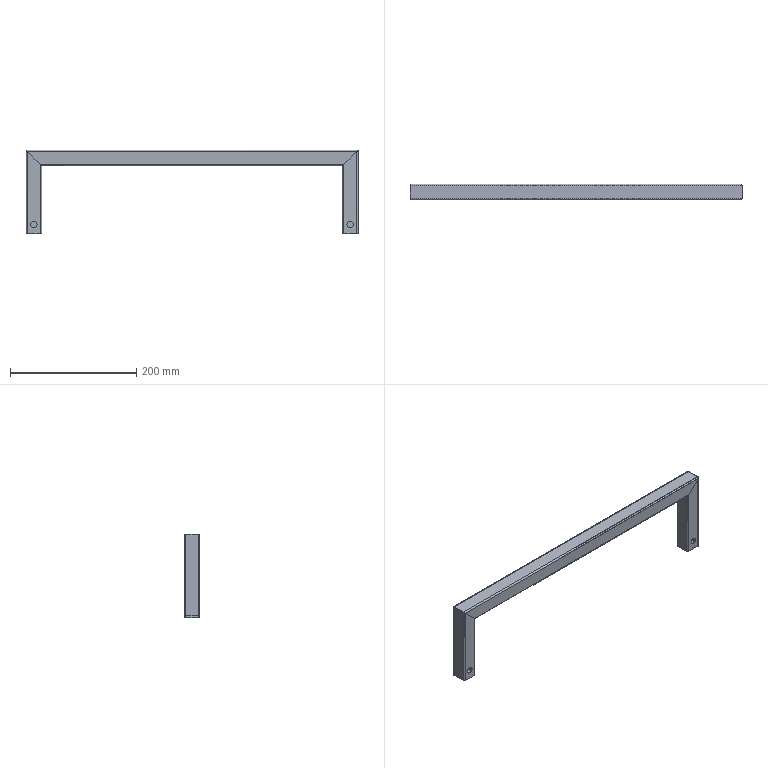Part | SolidWorks | features Cut 1, ICE 1, WeldMemberFeat 1, WeldmentFeature 1 | 3 solids | 60 faces | box 525 x 25 x 132.5 mm | volume 84662 mm3 | plane 32 | cylinder 28 | commonest cylinder face diameters 2.4 x12 4.8 x12 10 x4